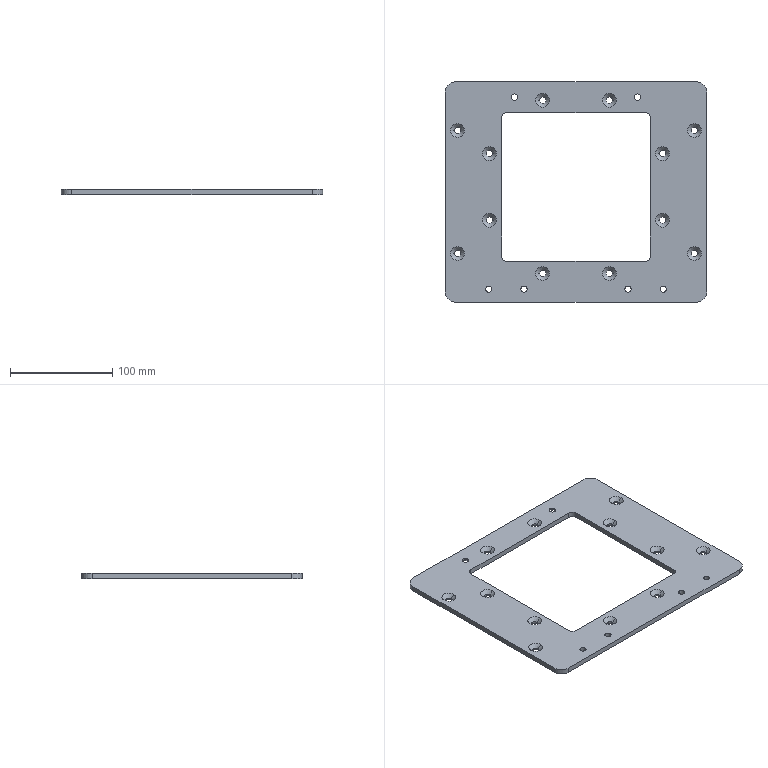Part | 1 solid | 82 faces | box 255 x 215 x 5 mm | volume 163410 mm3 | cylinder 44 | cone 28 | plane 10 | commonest cylinder face diameters 6.5 x28 6 x8 10 x4 20 x4